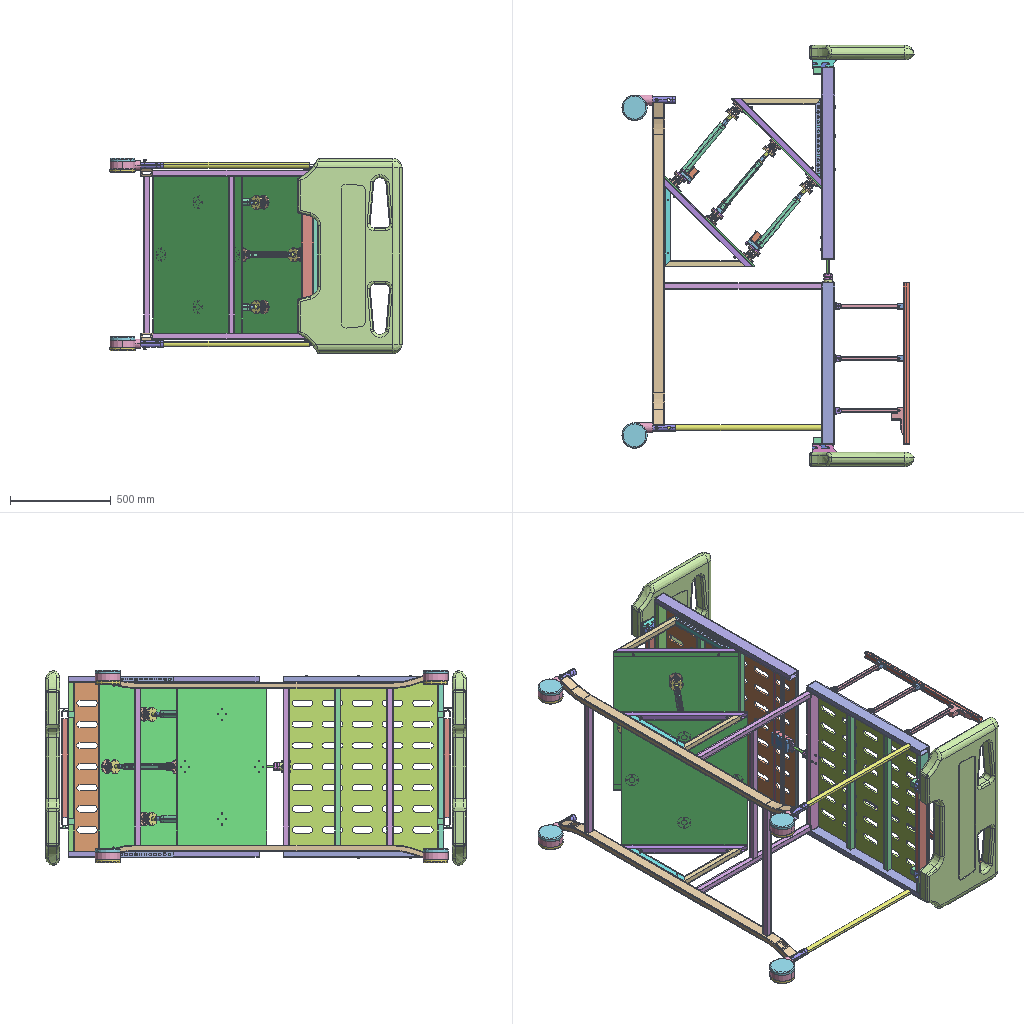Assembly | SolidWorks | 54 different items | 495 placed | box 1452 x 2094 x 971 mm
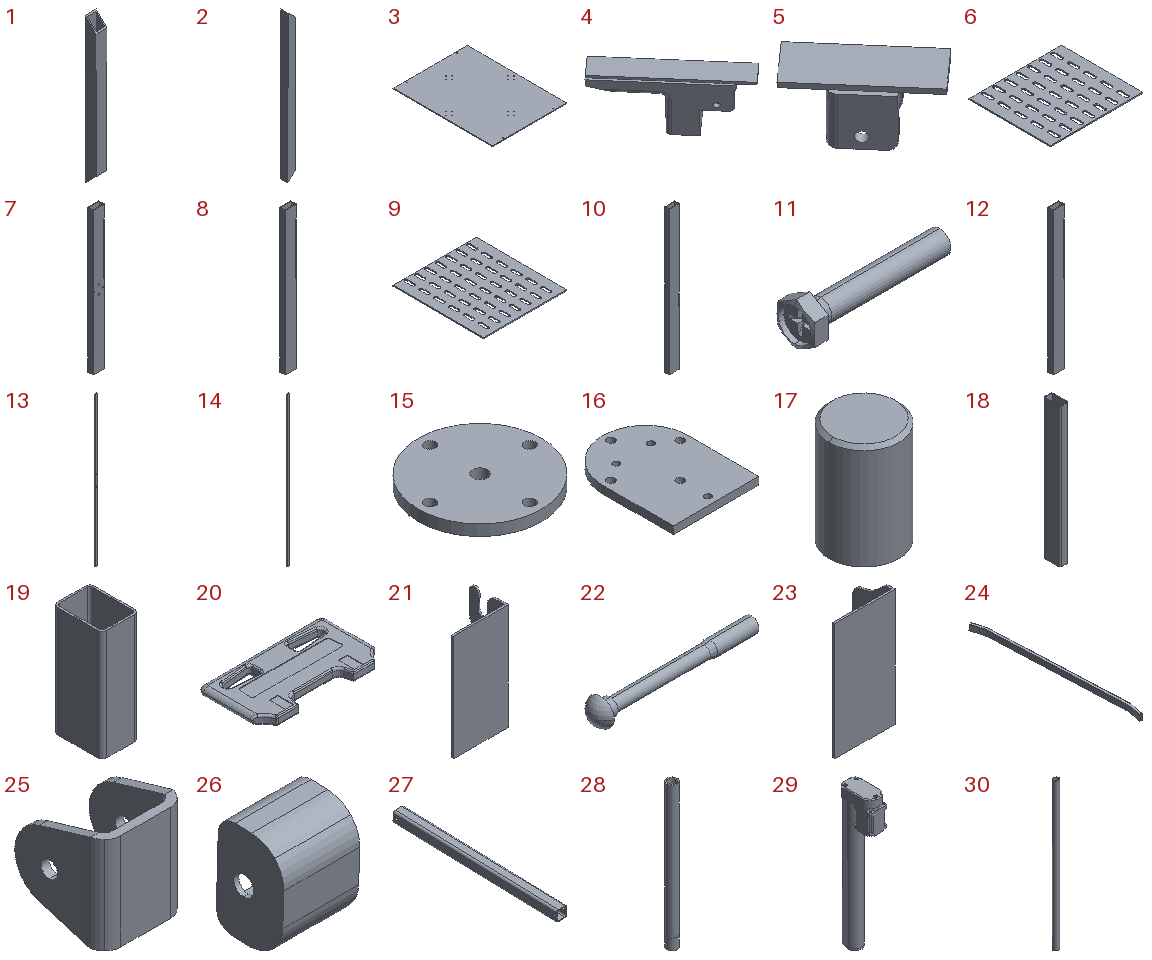Parts list (item | quantity | size | volume | features):
1 | x4 | 30 x 30 x 400 mm | 119880 mm3 | features ICE 3, Extrusion 1
2 | x4 | 30 x 30 x 625.685 mm | 192663 mm3 | features Cut 2, Extrusion 1, ICE 1
3 | x2 | 625.685 x 840 x 6 mm | 3151419 mm3 | features Cut 2, Extrusion 1
4 | x2 | 118.942 x 131.952 x 65.78 mm | 109548 mm3 | features BaseBody 1
5 | x4 | 64.897 x 69.371 x 35.986 mm | 22135 mm3 | features BaseBody 1
6 | x1 | 840 x 740 x 10 mm | 5160574 mm3 | features Extrusion 1, ICE 1
7 | x1 | 65 x 30 x 840 mm | 447881 mm3 | features ICE 2, Extrusion 1
8 | x1 | 65 x 30 x 840 mm | 448560 mm3 | features Extrusion 1, ICE 1
9 | x1 | 840 x 920 x 10 mm | 6461489 mm3 | features Extrusion 1, ICE 1
10 | x2 | 65 x 30 x 950 mm | 506395 mm3 | features Cut 1, Extrusion 1, ICE 1
11 | x24 | 39 x 10 x 11.547 mm | 1217 mm3 | features Cut 2, RevCut 2, CirPattern 1, Extrusion 1, LPattern 1, Revolution 1
12 | x1 | 65 x 30 x 840 mm | 448560 mm3 | features Extrusion 1, ICE 1
13 | x2 | 12 x 3 x 840 mm | 21761 mm3 | features 3DProfileFeature 1, Extrusion 1, HoleWzd 1, ICE 1
14 | x2 | 12 x 3 x 840 mm | 21840 mm3 | features Extrusion 1, ICE 1
15 | x4 | 68 x 68 x 6 mm | 21036 mm3 | features ICE 2, Extrusion 1
16 | x4 | 68 x 89.927 x 6 mm | 32907 mm3 | features Cut 2, Extrusion 1
17 | x8 | 10 x 10 x 15 mm | 1174 mm3 | features BaseBody 1
18 | x2 | 30 x 60 x 490 mm | 161830 mm3 | features BaseBody 1
19 | x4 | 30 x 40 x 90 mm | 17395 mm3 | features BaseBody 1
20 | x2 | 970 x 520 x 70 mm | 26489318 mm3 | features BaseBody 1
21 | x2 | 62 x 42 x 120 mm | 21824 mm3 | features BaseBody 1
22 | x6 | 85.28 x 14.328 x 14.328 mm | 3773 mm3 | features RevCut 2, LPattern 1, Revolution 1, Rib 1
23 | x2 | 62 x 42 x 120 mm | 21824 mm3 | features BaseBody 1
24 | x2 | 248.187 x 1610 x 188.463 mm | 531554 mm3 | features BaseBody 1
25 | x6 | 30 x 32.5 x 35 mm | 7224 mm3 | features BaseBody 1
26 | x6 | 23 x 20.424 x 30.136 mm | 5420 mm3 | features BaseBody 1
27 | x6 | 20 x 310.443 x 28.789 mm | 31845 mm3 | features BaseBody 1
28 | x4 | 20 x 20 x 284 mm | 37985 mm3 | features BaseBody 2
29 | x4 | 40 x 75.927 x 328 mm | 216478 mm3 | features BaseBody 20
30 | x2 | 28.9 x 28.9 x 840 mm | 105036 mm3 | features Extrusion 1
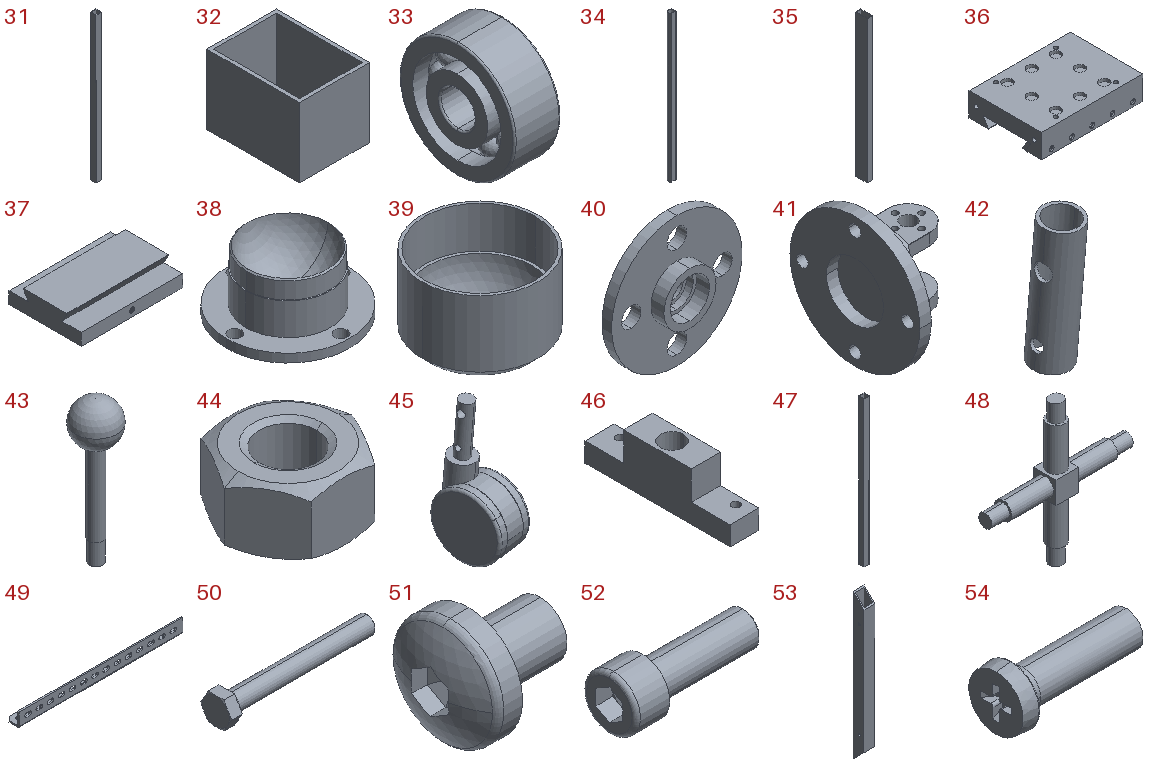31 | x5 | 30 x 30 x 784 mm | 254016 mm3 | features Extrusion 1
32 | x4 | 30 x 40 x 30 mm | 6030 mm3 | features Extrusion 1, ICE 1
33 | x32 | 4 x 10 x 10 mm | 208.039 mm3 | features Revolution 3, CirPattern 1, Fillet 1
34 | x2 | 30 x 30 x 800 mm | 132921 mm3 | features ICE 2, Extrusion 1
35 | x2 | 30 x 65 x 800 mm | 427200 mm3 | features Extrusion 1, ICE 1
36 | x1 | 105 x 75 x 24.5 mm | 146432 mm3 | features BaseBody 7, ICE 2
37 | x1 | 105 x 74.5 x 22 mm | 135687 mm3 | features BaseBody 1
38 | x1 | 58 x 58 x 27.375 mm | 26425 mm3 | features ICE 2, Extrusion 1, RevCut 1, StudWizard 1
39 | x1 | 42 x 42 x 27 mm | 6192 mm3 | features ICE 5, Chamfer 1, Extrusion 1, RevCut 1
40 | x32 | 20 x 3.5 x 20 mm | 446.892 mm3 | features ICE 1, Revolution 1
41 | x16 | 39 x 68 x 68 mm | 29102 mm3 | features ICE 8, MirrorPattern 2, Revolution 1
42 | x4 | 34.667 x 42.72 x 117.323 mm | 30652 mm3 | features BaseBody 1
43 | x1 | 38 x 38 x 130 mm | 40616 mm3 | features Revolution 2, StudWizard 1
44 | x33 | 9.238 x 8 x 4.7 mm | 190.603 mm3 | features RevCut 2, Chamfer 1, Extrusion 1, LPattern 1
45 | x4 | 83.862 x 131.58 x 256.05 mm | 967710 mm3 | features BaseBody 3
46 | x1 | 15 x 75 x 25 mm | 16595 mm3 | features Cut 3, Extrusion 1
47 | x4 | 30 x 30 x 840 mm | 272160 mm3 | features Extrusion 1, ICE 1
48 | x8 | 32 x 5 x 32 mm | 715.619 mm3 | features ICE 4, MirrorPattern 4, Extrusion 1
49 | x2 | 352 x 30 x 30 mm | 51066 mm3 | features ICE 3, Cut 1, Extrusion 1, Fillet 1
50 | x4 | 43.65 x 8.984 x 7.78 mm | 971.133 mm3 | features RevCut 3, Boss 1, Chamfer 1, Extrusion 1, Fillet 1, LPattern 1
51 | x4 | 12.382 x 12 x 12 mm | 602.281 mm3 | features Cut 2, Fillet 2, RevCut 2, Boss 1, Extrusion 1, LPattern 1
52 | x212 | 40 x 16 x 16 mm | 4032 mm3 | features Fillet 2, RevCut 2, Boss 1, Chamfer 1, Cut 1, Extrusion 1, LPattern 1
53 | x4 | 30 x 30 x 400 mm | 119541 mm3 | features ICE 4, Extrusion 1
54 | x2 | 11.4 x 4.982 x 4.982 mm | 94.532 mm3 | features Draft 2, Fillet 2, Boss 1, Cut 1, Extrusion 1, LPattern 1, PLine 1, RevCut 1
Mates (type | each side: item.copy, entity, surface, feature), first 538 of 1066 lines:
Coincident | 8.1 face plane Boss-Extrude1 | 35.1 face plane Boss-Extrude1 | 3 times
Coincident | 8.1 face plane Boss-Extrude1 | 35.2 face plane Boss-Extrude1 | 2 times
Coincident | 35.1 face plane Boss-Extrude1 | 35.2 face plane Boss-Extrude1
Coincident | 35.1 face plane Boss-Extrude1 | 47.1 face plane Boss-Extrude1
DistanceDim | 47.1 face plane Boss-Extrude1 | 35.1 face plane Boss-Extrude1
Coincident | 47.1 face plane Boss-Extrude1 | 47.2 face plane Boss-Extrude1
Coincident | 35.1 face plane Boss-Extrude1 | 47.2 face plane Boss-Extrude1
Coincident | 35.1 face plane Boss-Extrude1 | 7.1 face plane Boss-Extrude1 | 3 times
DistanceDim | 47.2 face plane Boss-Extrude1 | 7.1 face plane Boss-Extrude1
DistanceDim | 47.1 face plane Boss-Extrude1 | 8.1 face plane Boss-Extrude1
Coincident | 35.1 face plane Boss-Extrude1 | 25.1 face plane Guardrail support connector seat1^Guardrail bottom beam-6-solid1 | 2 times
DistanceDim | 25.1 face plane Guardrail support connector seat1^Guardrail bottom beam-6-solid1 | 8.1 face plane Boss-Extrude1
Coincident | 35.1 face plane Boss-Extrude1 | 25.2 face plane Guardrail support connector seat1^Guardrail bottom beam-6-solid1 | 2 times
DistanceDim | 25.2 face plane Guardrail support connector seat1^Guardrail bottom beam-6-solid1 | 8.1 face plane Boss-Extrude1
Coincident | 35.1 face plane Boss-Extrude1 | 25.3 face plane Guardrail support connector seat1^Guardrail bottom beam-6-solid1 | 2 times
DistanceDim | 25.3 face plane Guardrail support connector seat1^Guardrail bottom beam-6-solid1 | 8.1 face plane Boss-Extrude1
Coincident | 35.2 face plane Boss-Extrude1 | 25.4 face plane Guardrail support connector seat1^Guardrail bottom beam-6-solid1 | 2 times
Coincident | 25.1 face plane Guardrail support connector seat1^Guardrail bottom beam-6-solid1 | 25.4 face plane Guardrail support connector seat1^Guardrail bottom beam-6-solid1
Coincident | 35.2 face plane Boss-Extrude1 | 25.5 face plane Guardrail support connector seat1^Guardrail bottom beam-6-solid1 | 2 times
Coincident | 35.2 face plane Boss-Extrude1 | 25.6 face plane Guardrail support connector seat1^Guardrail bottom beam-6-solid1 | 2 times
Coincident | 25.2 face plane Guardrail support connector seat1^Guardrail bottom beam-6-solid1 | 25.5 face plane Guardrail support connector seat1^Guardrail bottom beam-6-solid1
Coincident | 25.3 face plane Guardrail support connector seat1^Guardrail bottom beam-6-solid1 | 25.6 face plane Guardrail support connector seat1^Guardrail bottom beam-6-solid1
Concentric | 25.1 face cylinder Guardrail support connector seat1^Guardrail bottom beam-6-solid1 | 26.1 face cylinder Nylon seat1^Guardrail assembly-6-solid1
Parallel | 25.1 face plane Guardrail support connector seat1^Guardrail bottom beam-6-solid1 | 26.1 face plane Nylon seat1^Guardrail assembly-6-solid1
Coincident | 25.1 face plane Guardrail support connector seat1^Guardrail bottom beam-6-solid1 | 26.1 face plane Nylon seat1^Guardrail assembly-6-solid1
Concentric | 25.2 face cylinder Guardrail support connector seat1^Guardrail bottom beam-6-solid1 | 26.2 face cylinder Nylon seat1^Guardrail assembly-6-solid1
Parallel | 25.2 face plane Guardrail support connector seat1^Guardrail bottom beam-6-solid1 | 26.2 face plane Nylon seat1^Guardrail assembly-6-solid1
Coincident | 25.2 face plane Guardrail support connector seat1^Guardrail bottom beam-6-solid1 | 26.2 face plane Nylon seat1^Guardrail assembly-6-solid1
Concentric | 25.3 face cylinder Guardrail support connector seat1^Guardrail bottom beam-6-solid1 | 26.3 face cylinder Nylon seat1^Guardrail assembly-6-solid1
Parallel | 25.3 face plane Guardrail support connector seat1^Guardrail bottom beam-6-solid1 | 26.3 face plane Nylon seat1^Guardrail assembly-6-solid1
Coincident | 25.3 face plane Guardrail support connector seat1^Guardrail bottom beam-6-solid1 | 26.3 face plane Nylon seat1^Guardrail assembly-6-solid1
Concentric | 25.4 face cylinder Guardrail support connector seat1^Guardrail bottom beam-6-solid1 | 26.4 face cylinder Nylon seat1^Guardrail assembly-6-solid1
Parallel | 25.4 face plane Guardrail support connector seat1^Guardrail bottom beam-6-solid1 | 26.4 face plane Nylon seat1^Guardrail assembly-6-solid1
Coincident | 25.4 face plane Guardrail support connector seat1^Guardrail bottom beam-6-solid1 | 26.4 face plane Nylon seat1^Guardrail assembly-6-solid1
Concentric | 25.5 face cylinder Guardrail support connector seat1^Guardrail bottom beam-6-solid1 | 26.5 face cylinder Nylon seat1^Guardrail assembly-6-solid1
Parallel | 25.5 face plane Guardrail support connector seat1^Guardrail bottom beam-6-solid1 | 26.5 face plane Nylon seat1^Guardrail assembly-6-solid1
Coincident | 25.5 face plane Guardrail support connector seat1^Guardrail bottom beam-6-solid1 | 26.5 face plane Nylon seat1^Guardrail assembly-6-solid1
Concentric | 25.6 face cylinder Guardrail support connector seat1^Guardrail bottom beam-6-solid1 | 26.6 face cylinder Nylon seat1^Guardrail assembly-6-solid1
Parallel | 25.6 face plane Guardrail support connector seat1^Guardrail bottom beam-6-solid1 | 26.6 face plane Nylon seat1^Guardrail assembly-6-solid1
Coincident | 25.6 face plane Guardrail support connector seat1^Guardrail bottom beam-6-solid1 | 26.6 face plane Nylon seat1^Guardrail assembly-6-solid1
Concentric | 25.1 face cylinder Guardrail support connector seat1^Guardrail bottom beam-6-solid1 | 27.1 face cylinder Steel F 20x20x1.5-310 GB_T 6728-2002^Guardrail assembly-3-solid1
Parallel | 35.1 face plane Boss-Extrude1 | 27.1 face plane Steel F 20x20x1.5-310 GB_T 6728-2002^Guardrail assembly-3-solid1
Coincident | 26.1 face plane Nylon seat1^Guardrail assembly-6-solid1 | 27.1 face plane Steel F 20x20x1.5-310 GB_T 6728-2002^Guardrail assembly-3-solid1
Concentric | 25.2 face cylinder Guardrail support connector seat1^Guardrail bottom beam-6-solid1 | 27.2 face cylinder Steel F 20x20x1.5-310 GB_T 6728-2002^Guardrail assembly-3-solid1
Parallel | 35.1 face plane Boss-Extrude1 | 27.2 face plane Steel F 20x20x1.5-310 GB_T 6728-2002^Guardrail assembly-3-solid1
Coincident | 26.2 face plane Nylon seat1^Guardrail assembly-6-solid1 | 27.2 face plane Steel F 20x20x1.5-310 GB_T 6728-2002^Guardrail assembly-3-solid1
Concentric | 25.3 face cylinder Guardrail support connector seat1^Guardrail bottom beam-6-solid1 | 27.3 face cylinder Steel F 20x20x1.5-310 GB_T 6728-2002^Guardrail assembly-3-solid1
Parallel | 35.1 face plane Boss-Extrude1 | 27.3 face plane Steel F 20x20x1.5-310 GB_T 6728-2002^Guardrail assembly-3-solid1
Coincident | 26.3 face plane Nylon seat1^Guardrail assembly-6-solid1 | 27.3 face plane Steel F 20x20x1.5-310 GB_T 6728-2002^Guardrail assembly-3-solid1
Concentric | 25.4 face cylinder Guardrail support connector seat1^Guardrail bottom beam-6-solid1 | 27.4 face cylinder Steel F 20x20x1.5-310 GB_T 6728-2002^Guardrail assembly-3-solid1
Parallel | 35.2 face plane Boss-Extrude1 | 27.4 face plane Steel F 20x20x1.5-310 GB_T 6728-2002^Guardrail assembly-3-solid1
Concentric | 25.5 face cylinder Guardrail support connector seat1^Guardrail bottom beam-6-solid1 | 27.5 face cylinder Steel F 20x20x1.5-310 GB_T 6728-2002^Guardrail assembly-3-solid1
Parallel | 35.2 face plane Boss-Extrude1 | 27.5 face plane Steel F 20x20x1.5-310 GB_T 6728-2002^Guardrail assembly-3-solid1
Coincident | 26.5 face plane Nylon seat1^Guardrail assembly-6-solid1 | 27.5 face plane Steel F 20x20x1.5-310 GB_T 6728-2002^Guardrail assembly-3-solid1
Concentric | 26.6 face cylinder Nylon seat1^Guardrail assembly-6-solid1 | 27.6 face cylinder Steel F 20x20x1.5-310 GB_T 6728-2002^Guardrail assembly-3-solid1
Parallel | 35.2 face plane Boss-Extrude1 | 27.6 face plane Steel F 20x20x1.5-310 GB_T 6728-2002^Guardrail assembly-3-solid1
Coincident | 26.6 face plane Nylon seat1^Guardrail assembly-6-solid1 | 27.6 face plane Steel F 20x20x1.5-310 GB_T 6728-2002^Guardrail assembly-3-solid1
Concentric | 27.4 face cylinder Steel F 20x20x1.5-310 GB_T 6728-2002^Guardrail assembly-3-solid1 | 4.1 face cylinder Nylon seat3^Upper crossbeam assembly-1-solid1
Parallel | 35.2 face plane Boss-Extrude1 | 4.1 face plane Nylon seat3^Upper crossbeam assembly-1-solid1
Coincident | 27.4 face plane Steel F 20x20x1.5-310 GB_T 6728-2002^Guardrail assembly-3-solid1 | 4.1 face plane Nylon seat3^Upper crossbeam assembly-1-solid1
Coincident | 26.4 face plane Nylon seat1^Guardrail assembly-6-solid1 | 27.4 face plane Steel F 20x20x1.5-310 GB_T 6728-2002^Guardrail assembly-3-solid1
Concentric | 27.1 face cylinder Steel F 20x20x1.5-310 GB_T 6728-2002^Guardrail assembly-3-solid1 | 4.2 face cylinder Nylon seat3^Upper crossbeam assembly-1-solid1
Parallel | 35.1 face plane Boss-Extrude1 | 4.2 face plane Nylon seat3^Upper crossbeam assembly-1-solid1
Coincident | 27.1 face plane Steel F 20x20x1.5-310 GB_T 6728-2002^Guardrail assembly-3-solid1 | 4.2 face plane Nylon seat3^Upper crossbeam assembly-1-solid1
Concentric | 27.5 face cylinder Steel F 20x20x1.5-310 GB_T 6728-2002^Guardrail assembly-3-solid1 | 5.1 face cylinder Nylon seat2^Upper crossbeam assembly-4-solid1
Parallel | 35.2 face plane Boss-Extrude1 | 5.1 face plane Nylon seat2^Upper crossbeam assembly-4-solid1
Coincident | 27.5 face plane Steel F 20x20x1.5-310 GB_T 6728-2002^Guardrail assembly-3-solid1 | 5.1 face plane Nylon seat2^Upper crossbeam assembly-4-solid1
Concentric | 27.6 face cylinder Steel F 20x20x1.5-310 GB_T 6728-2002^Guardrail assembly-3-solid1 | 5.2 face cylinder Nylon seat2^Upper crossbeam assembly-4-solid1
Parallel | 35.2 face plane Boss-Extrude1 | 5.2 face plane Nylon seat2^Upper crossbeam assembly-4-solid1
Coincident | 27.6 face plane Steel F 20x20x1.5-310 GB_T 6728-2002^Guardrail assembly-3-solid1 | 5.2 face plane Nylon seat2^Upper crossbeam assembly-4-solid1
Concentric | 27.2 face cylinder Steel F 20x20x1.5-310 GB_T 6728-2002^Guardrail assembly-3-solid1 | 5.3 face cylinder Nylon seat2^Upper crossbeam assembly-4-solid1
Parallel | 35.1 face plane Boss-Extrude1 | 5.3 face plane Nylon seat2^Upper crossbeam assembly-4-solid1
Coincident | 27.2 face plane Steel F 20x20x1.5-310 GB_T 6728-2002^Guardrail assembly-3-solid1 | 5.3 face plane Nylon seat2^Upper crossbeam assembly-4-solid1
Concentric | 27.3 face cylinder Steel F 20x20x1.5-310 GB_T 6728-2002^Guardrail assembly-3-solid1 | 5.4 face cylinder Nylon seat2^Upper crossbeam assembly-4-solid1
Parallel | 35.1 face plane Boss-Extrude1 | 5.4 face plane Nylon seat2^Upper crossbeam assembly-4-solid1
Coincident | 27.3 face plane Steel F 20x20x1.5-310 GB_T 6728-2002^Guardrail assembly-3-solid1 | 5.4 face plane Nylon seat2^Upper crossbeam assembly-4-solid1
Coincident | 4.2 face plane Nylon seat3^Upper crossbeam assembly-1-solid1 | 34.1 face plane Cut-Extrude2 | 2 times
Coincident | 35.1 face plane Boss-Extrude1 | 34.1 face plane Boss-Extrude1
Coincident | 4.1 face plane Nylon seat3^Upper crossbeam assembly-1-solid1 | 34.2 face plane Cut-Extrude2 | 2 times
Coincident | 35.2 face plane Boss-Extrude1 | 34.2 face plane Boss-Extrude1
Concentric | 5.4 face cylinder Nylon seat2^Upper crossbeam assembly-4-solid1 | 11.1 face cylinder Revolve1
Coincident | 5.4 face plane Nylon seat2^Upper crossbeam assembly-4-solid1 | 11.1 face plane BaseHead
Concentric | 25.3 face cylinder Guardrail support connector seat1^Guardrail bottom beam-6-solid1 | 11.2 face cylinder Revolve1
Coincident | 25.3 face plane Guardrail support connector seat1^Guardrail bottom beam-6-solid1 | 11.2 face plane BaseHead
Concentric | 25.2 face cylinder Guardrail support connector seat1^Guardrail bottom beam-6-solid1 | 11.3 face cylinder Revolve1
Concentric | 5.3 face cylinder Nylon seat2^Upper crossbeam assembly-4-solid1 | 11.4 face cylinder Revolve1
Concentric | 25.1 face cylinder Guardrail support connector seat1^Guardrail bottom beam-6-solid1 | 11.5 face cylinder Revolve1
Concentric | 4.2 face cylinder Nylon seat3^Upper crossbeam assembly-1-solid1 | 11.6 face cylinder Revolve1
Coincident | 25.2 face plane Guardrail support connector seat1^Guardrail bottom beam-6-solid1 | 11.3 face plane BaseHead
Coincident | 5.3 face plane Nylon seat2^Upper crossbeam assembly-4-solid1 | 11.4 face plane BaseHead
Coincident | 25.1 face plane Guardrail support connector seat1^Guardrail bottom beam-6-solid1 | 11.5 face plane BaseHead
Coincident | 4.2 face plane Nylon seat3^Upper crossbeam assembly-1-solid1 | 11.6 face plane BaseHead
Concentric | 25.6 face cylinder Guardrail support connector seat1^Guardrail bottom beam-6-solid1 | 11.7 face cylinder Revolve1
Coincident | 25.6 face plane Guardrail support connector seat1^Guardrail bottom beam-6-solid1 | 11.7 face plane BaseHead
Concentric | 5.2 face cylinder Nylon seat2^Upper crossbeam assembly-4-solid1 | 11.8 face cylinder Revolve1
Coincident | 5.2 face plane Nylon seat2^Upper crossbeam assembly-4-solid1 | 11.8 face plane BaseHead
Concentric | 25.5 face cylinder Guardrail support connector seat1^Guardrail bottom beam-6-solid1 | 11.9 face cylinder Revolve1
Coincident | 25.5 face plane Guardrail support connector seat1^Guardrail bottom beam-6-solid1 | 11.9 face plane BaseHead
Concentric | 5.1 face cylinder Nylon seat2^Upper crossbeam assembly-4-solid1 | 11.10 face cylinder Revolve1
Coincident | 5.1 face plane Nylon seat2^Upper crossbeam assembly-4-solid1 | 11.10 face plane BaseHead
Concentric | 4.1 face cylinder Nylon seat3^Upper crossbeam assembly-1-solid1 | 11.11 face cylinder Revolve1
Coincident | 4.1 face plane Nylon seat3^Upper crossbeam assembly-1-solid1 | 11.11 face plane BaseHead
Concentric | 25.4 face cylinder Guardrail support connector seat1^Guardrail bottom beam-6-solid1 | 11.12 face cylinder Revolve1
Coincident | 25.4 face plane Guardrail support connector seat1^Guardrail bottom beam-6-solid1 | 11.12 face plane BaseHead
Concentric | 11.7 face cylinder Revolve1 | 44.1 face cylinder BaseNut
Concentric | 11.8 face cylinder Revolve1 | 44.2 face cylinder BaseNut
Concentric | 11.9 face cylinder Revolve1 | 44.3 face cylinder BaseNut
Concentric | 11.10 face cylinder Revolve1 | 44.4 face cylinder BaseNut
Concentric | 11.12 face cylinder Revolve1 | 44.5 face cylinder BaseNut
Concentric | 11.11 face cylinder Revolve1 | 44.6 face cylinder BaseNut
Coincident | 25.4 face plane Guardrail support connector seat1^Guardrail bottom beam-6-solid1 | 44.5 face plane BaseNut
Coincident | 4.1 face plane Nylon seat3^Upper crossbeam assembly-1-solid1 | 44.6 face plane BaseNut
Coincident | 5.1 face plane Nylon seat2^Upper crossbeam assembly-4-solid1 | 44.4 face plane BaseNut
Coincident | 25.5 face plane Guardrail support connector seat1^Guardrail bottom beam-6-solid1 | 44.3 face plane BaseNut
Coincident | 25.6 face plane Guardrail support connector seat1^Guardrail bottom beam-6-solid1 | 44.1 face plane BaseNut
Concentric | 11.1 face cylinder Revolve1 | 44.7 face cylinder BaseNut
Concentric | 11.4 face cylinder Revolve1 | 44.8 face cylinder BaseNut
Concentric | 11.6 face cylinder Revolve1 | 44.9 face cylinder BaseNut
Coincident | 4.2 face plane Nylon seat3^Upper crossbeam assembly-1-solid1 | 44.9 face plane BaseNut
Concentric | 11.5 face cylinder Revolve1 | 44.10 face cylinder BaseNut
Coincident | 25.1 face plane Guardrail support connector seat1^Guardrail bottom beam-6-solid1 | 44.10 face plane BaseNut
Concentric | 11.3 face cylinder Revolve1 | 44.11 face cylinder BaseNut
Coincident | 5.3 face plane Nylon seat2^Upper crossbeam assembly-4-solid1 | 44.8 face plane BaseNut
Coincident | 25.2 face plane Guardrail support connector seat1^Guardrail bottom beam-6-solid1 | 44.11 face plane BaseNut
Concentric | 11.2 face cylinder Revolve1 | 44.12 face cylinder BaseNut
Coincident | 25.3 face plane Guardrail support connector seat1^Guardrail bottom beam-6-solid1 | 44.12 face plane BaseNut
Coincident | 5.4 face plane Nylon seat2^Upper crossbeam assembly-4-solid1 | 44.7 face plane BaseNut
Coincident | 7.1 face plane Boss-Extrude1 | 38.1 face plane Boss-Extrude1
Concentric | 7.1 face cylinder Cut-Extrude3 | 38.1 face cylinder Cut-Extrude1 | 2 times
Concentric | 38.1 face sphere Cut-Revolve4 | 43.1 face sphere Revolve5
Concentric | 38.1 face cylinder Boss-Extrude2 | 43.1 face cylinder Revolve6
Concentric | 38.1 face cylinder Boss-Extrude2 | 39.1 face cylinder Boss-Extrude1
Coincident | 38.1 face plane M39 mechanical thread stud1 | 39.1 face plane Boss-Extrude1
Concentric | 43.1 face cylinder Revolve6 | 46.1 face cylinder Cut-Extrude3
Coincident | 43.1 face plane M12x1.25 mechanical thread stud1 | 46.1 face plane Boss-Extrude1
Concentric | 46.1 face cylinder Cut-Extrude1 | 36.1 face cylinder 21060_TOP^COMPANY_A_21060-075105.step-1-solid1 | 2 times
Coincident | 46.1 face plane Boss-Extrude1 | 36.1 face plane 21060_TOP^COMPANY_A_21060-075105.step-1-solid1
Lock | 10.1 select_type:0 | 12.1 select_type:0
Lock | 10.2 select_type:0 | 12.1 select_type:0
Coincident | 37.1 face plane 21060_BOTTOM^COMPANY_A_21060-075105.step-1-solid1 | 36.1 face plane 21060_TOP^COMPANY_A_21060-075105.step-1-solid1 | 2 times
Coincident | 37.1 face plane 21060_BOTTOM^COMPANY_A_21060-075105.step-1-solid1 | 36.1 face plane 21060_TOP^COMPANY_A_21060-075105.step-1-solid2
Parallel | 7.1 face plane Boss-Extrude1 | 36.1 face plane Boss-Extrude1
Coincident | 10.2 face plane Boss-Extrude1 | 46.1 face plane Boss-Extrude1
Coincident | 35.1 face plane Boss-Extrude1 | 10.2 face plane Boss-Extrude1 | 2 times
Concentric | 37.1 face cylinder 21060_BOTTOM^COMPANY_A_21060-075105.step-1-solid1 | 13.1 face cylinder M6 Tapped Hole1 | 2 times
Coincident | 10.1 face plane Boss-Extrude1 | 13.1 face plane Boss-Extrude1
Concentric | 37.1 face cylinder 21060_BOTTOM^COMPANY_A_21060-075105.step-1-solid1 | 13.2 face cylinder M6 Tapped Hole1 | 2 times
Coincident | 10.2 face plane Boss-Extrude1 | 13.2 face plane Boss-Extrude1
Coincident | 10.2 face plane Boss-Extrude1 | 47.3 face plane Boss-Extrude1
DistanceDim | 47.3 face plane Boss-Extrude1 | 10.2 face plane Boss-Extrude1
Coincident | 10.2 face plane Boss-Extrude1 | 47.4 face plane Boss-Extrude1
DistanceDim | 47.4 face plane Boss-Extrude1 | 10.2 face plane Boss-Extrude1
DistanceDim | 47.3 face plane Boss-Extrude1 | 12.1 face plane Boss-Extrude1
DistanceDim | 47.4 face plane Boss-Extrude1 | 37.1 face plane 21060_BOTTOM^COMPANY_A_21060-075105.step-1-solid1
Coincident | 20.1 face plane Input1 | 21.1 face plane Input1 | 3 times
Coincident | 20.1 face plane Input1 | 23.1 face plane Input1 | 3 times
Concentric | 23.1 face cylinder Input1 | 17.1 face cylinder Input1
Coincident | 23.1 face plane Input1 | 17.1 face plane Input1
Concentric | 23.1 face cylinder Input1 | 17.2 face cylinder Input1
Coincident | 17.2 face plane Input1 | 17.1 face plane Input1
Concentric | 21.1 face cylinder Input1 | 17.3 face cylinder Input1
Coincident | 21.1 face plane Input1 | 17.3 face plane Input1
DistanceDim | 19.1 face plane Input1 | 21.1 face plane Input1 | 2 times
Concentric | 21.1 face cylinder Input1 | 17.4 face cylinder Input1
Coincident | 17.3 face plane Input1 | 17.4 face plane Input1
Coincident | 19.1 face plane Input1 | 19.2 face plane Input1
Coincident | 19.1 face plane Input1 | 18.1 face plane Input1 | 3 times
Coincident | 18.1 face plane Input1 | 19.2 face plane Input1 | 2 times
Coincident | 20.1 face plane Input1 | 19.1 face plane Input1
DistanceDim | 19.2 face plane Input1 | 18.1 face plane Input1
Coincident | 23.2 face plane Input1 | 20.2 face plane Input1 | 3 times
Coincident | 21.2 face plane Input1 | 20.2 face plane Input1 | 3 times
DistanceDim | 19.3 face plane Input1 | 21.2 face plane Input1 | 2 times
Concentric | 17.5 face cylinder Input1 | 23.2 face cylinder Input1
Concentric | 17.6 face cylinder Input1 | 21.2 face cylinder Input1
Concentric | 17.7 face cylinder Input1 | 23.2 face cylinder Input1
Concentric | 17.8 face cylinder Input1 | 21.2 face cylinder Input1
DistanceDim | 19.4 face plane Input1 | 18.2 face plane Input1
Coincident | 18.2 face plane Input1 | 19.3 face plane Input1 | 3 times
Coincident | 19.4 face plane Input1 | 19.3 face plane Input1
Coincident | 17.6 face plane Input1 | 17.8 face plane Input1
Coincident | 18.2 face plane Input1 | 19.4 face plane Input1 | 2 times
Coincident | 19.3 face plane Input1 | 20.2 face plane Input1
Coincident | 17.7 face plane Input1 | 17.5 face plane Input1
Coincident | 17.5 face plane Input1 | 23.2 face plane Input1
Coincident | 17.8 face plane Input1 | 21.2 face plane Input1
Coincident | 19.3 face plane Input1 | 32.1 face plane Boss-Extrude1
Coincident | 19.3 edge | 32.1 face plane Boss-Extrude1
Coincident | 18.2 face plane Input1 | 32.1 face plane Boss-Extrude1
Coincident | 19.4 face plane Input1 | 32.2 face plane Boss-Extrude1
Coincident | 19.4 edge | 32.2 face plane Boss-Extrude1
Coincident | 32.1 face plane Boss-Extrude1 | 32.2 face plane Boss-Extrude1
Coincident | 8.1 face plane Boss-Extrude1 | 32.2 face plane Boss-Extrude1
Coincident | 8.1 face plane Boss-Extrude1 | 19.3 face plane Input1
DistanceDim | 21.2 face plane Input1 | 35.2 face plane Boss-Extrude1
Coincident | 19.1 face plane Input1 | 32.3 face plane Boss-Extrude1
Coincident | 19.1 edge | 32.3 face plane Boss-Extrude1
Coincident | 18.1 face plane Input1 | 32.3 face plane Boss-Extrude1
Coincident | 19.2 face plane Input1 | 32.4 face plane Boss-Extrude1
Coincident | 19.2 edge | 32.4 face plane Boss-Extrude1
Coincident | 32.3 face plane Boss-Extrude1 | 32.4 face plane Boss-Extrude1
Coincident | 12.1 face plane Boss-Extrude1 | 32.3 face plane Boss-Extrude1
Coincident | 32.1 face plane Boss-Extrude1 | 32.4 face plane Boss-Extrude1
Coincident | 12.1 face plane Boss-Extrude1 | 19.2 face plane Input1
Coincident | 10.2 face plane Boss-Extrude1 | 14.1 face plane Boss-Extrude1
Coincident | 13.2 face plane Boss-Extrude1 | 14.1 face plane Boss-Extrude1
Coincident | 10.2 face plane Boss-Extrude1 | 14.2 face plane Boss-Extrude1
Coincident | 10.1 face plane Boss-Extrude1 | 14.2 face plane Boss-Extrude1
Coincident | 10.2 face plane Boss-Extrude1 | 9.1 face plane Boss-Extrude1 | 2 times
Coincident | 12.1 face plane Boss-Extrude1 | 9.1 face plane Boss-Extrude1
Coincident | 35.1 face plane Boss-Extrude1 | 6.1 face plane Boss-Extrude1 | 2 times
Coincident | 7.1 face plane Boss-Extrude1 | 6.1 face plane Boss-Extrude1
Concentric | 38.1 face cylinder Cut-Extrude1 | 50.1 face cylinder BaseBody
Coincident | 38.1 face plane Boss-Extrude1 | 50.1 face plane BearingFace
Concentric | 38.1 face cylinder Cut-Extrude1 | 50.2 face cylinder BaseBody
Coincident | 50.1 face plane BaseHead | 50.2 face plane BaseHead
Concentric | 38.1 face cylinder Cut-Extrude1 | 50.3 face cylinder BaseBody
Coincident | 50.2 face plane BaseHead | 50.3 face plane BaseHead
Concentric | 38.1 face cylinder Cut-Extrude1 | 50.4 face cylinder BaseBody
Coincident | 50.1 face plane BaseHead | 50.4 face plane BaseHead
Coincident | 7.1 face plane Boss-Extrude1 | 44.13 face plane BaseNut
Concentric | 50.4 face cylinder BaseBody | 44.13 face cylinder BaseNut
Concentric | 50.2 face cylinder BaseBody | 44.14 face cylinder BaseNut
Coincident | 44.14 face plane BaseNut | 44.13 face plane BaseNut
Concentric | 50.3 face cylinder BaseBody | 44.15 face cylinder BaseNut
Coincident | 44.15 face plane BaseNut | 44.13 face plane BaseNut
Coincident | 13.1 face plane Boss-Extrude1 | 51.1 face plane BaseHead
Coincident | 13.1 face plane Boss-Extrude1 | 51.2 face plane BaseHead
Coincident | 13.2 face plane Boss-Extrude1 | 51.3 face plane BaseHead
Coincident | 13.2 face plane Boss-Extrude1 | 51.4 face plane BaseHead
Concentric | 13.1 face cylinder M6 Tapped Hole1 | 51.1 face cylinder BaseBody
Concentric | 13.1 edge | 51.2 face cylinder BaseHead
Concentric | 13.2 edge | 51.4 face cylinder BaseHead
Concentric | 13.2 face cylinder M6 Tapped Hole1 | 51.3 face cylinder BaseHead
Concentric | 46.1 face cylinder Cut-Extrude1 | 54.1 face cone SplitLine1
Coincident | 46.1 face plane Cut-Extrude2 | 54.1 face plane BaseHead
Coincident | 46.1 face plane Cut-Extrude2 | 54.2 face plane BaseHead
Concentric | 46.1 face cylinder Cut-Extrude1 | 54.2 face cylinder SplitLine1
Coincident | 10.2 face plane Boss-Extrude1 | 49.1 face plane Boss-Extrude2 | 2 times
Coincident | 53.1 face plane Cut-Extrude3 | 1.1 face plane Cut-Extrude6
Coincident | 53.1 face plane Boss-Extrude1 | 1.1 face plane Boss-Extrude1
Coincident | 53.1 face plane Boss-Extrude1 | 1.1 edge
Coincident | 53.1 face plane Cut-Extrude6 | 2.1 face plane Boss-Extrude1
Coincident | 1.1 face plane Cut-Extrude3 | 2.1 face plane Boss-Extrude1
Coincident | 1.1 face plane Boss-Extrude1 | 2.1 face plane Boss-Extrude1
Coincident | 1.1 face plane Boss-Extrude1 | 2.1 face plane Cut-Extrude2
Coincident | 49.1 face plane Boss-Extrude1 | 53.1 face plane Boss-Extrude1
Coincident | 10.2 face plane Boss-Extrude1 | 53.1 face plane Boss-Extrude1
Lock | 49.1 select_type:0 | 53.1 select_type:0
DistanceDim | 1.1 face plane Boss-Extrude1 | 12.1 face plane Boss-Extrude1
Coincident | 14.1 face plane Boss-Extrude1 | 9.1 face plane Boss-Extrude1
Coincident | 14.2 face plane Boss-Extrude1 | 9.1 face plane Boss-Extrude1
Coincident | 10.1 face plane Boss-Extrude1 | 49.2 face plane Boss-Extrude2 | 2 times
Coincident | 49.1 face plane Boss-Extrude1 | 49.2 face plane Boss-Extrude1
Coincident | 53.2 face plane Cut-Extrude6 | 1.2 face plane Cut-Extrude6
Coincident | 53.2 face plane Boss-Extrude1 | 1.2 edge
Coincident | 53.2 face plane Boss-Extrude1 | 1.2 face plane Boss-Extrude1
Coincident | 53.2 face plane Cut-Extrude3 | 2.2 face plane Boss-Extrude1
Coincident | 53.2 face plane Boss-Extrude1 | 2.2 face plane Boss-Extrude1
Coincident | 1.2 face plane Boss-Extrude1 | 2.2 face plane Cut-Extrude2
Coincident | 49.2 face plane Boss-Extrude1 | 53.2 face plane Boss-Extrude1
Coincident | 10.1 face plane Boss-Extrude1 | 53.2 face plane Boss-Extrude1
Coincident | 1.1 face plane Boss-Extrude1 | 1.2 face plane Boss-Extrude1
InPlace | 2.2 face plane Boss-Extrude1 | 3.1 plane
Concentric | 10.2 face cylinder Cut-Extrude2 | 22.1 face cylinder Base
Coincident | 10.2 face plane Boss-Extrude1 | 22.1 face plane Base
Concentric | 10.2 face cylinder Cut-Extrude2 | 22.2 face cylinder Cut-Revolve1
Concentric | 10.2 face cylinder Cut-Extrude2 | 22.3 face cylinder Cut-Revolve1
Concentric | 10.1 face cylinder Cut-Extrude2 | 22.4 face cylinder Cut-Revolve1
Concentric | 10.1 face cylinder Cut-Extrude2 | 22.5 face cylinder Cut-Revolve1
Concentric | 10.1 face cylinder Cut-Extrude2 | 22.6 face cylinder Cut-Revolve1
Coincident | 22.2 face plane Base | 22.1 face plane Base
Coincident | 22.2 face plane Base | 22.3 face plane Base
Coincident | 22.1 face plane Base | 22.5 face plane Base
Coincident | 22.5 face plane Base | 22.6 face plane Base
Coincident | 22.5 face plane Base | 22.4 face plane Base
Concentric | 22.2 face cylinder Base | 44.16 face cylinder BaseNut
Concentric | 10.1 face cylinder Cut-Extrude2 | 44.17 face cone EndChamfer
Coincident | 10.1 face plane Boss-Extrude1 | 44.17 face plane BaseNut
Concentric | 22.4 face cylinder Base | 44.18 face cylinder BaseNut
Concentric | 22.5 face cylinder Base | 44.19 face cylinder BaseNut
Concentric | 22.1 face cylinder Base | 44.20 face cylinder BaseNut
Concentric | 22.3 face cylinder Base | 44.21 face cylinder BaseNut
Concentric | 3.1 face cylinder Cut-Extrude2 | 11.13 face cylinder Revolve1
Coincident | 3.1 face plane Boss-Extrude1 | 11.13 face plane BaseHead
Concentric | 3.1 face cylinder Cut-Extrude2 | 11.14 face cylinder Revolve1
Coincident | 3.1 face plane Boss-Extrude1 | 11.14 face plane BaseHead
Concentric | 3.1 face cylinder Cut-Extrude2 | 11.15 face cylinder Revolve1
Coincident | 3.1 face plane Boss-Extrude1 | 11.15 face plane BaseHead
Concentric | 3.1 face cylinder Cut-Extrude2 | 11.16 face cylinder Revolve1
Coincident | 3.1 face plane Boss-Extrude1 | 11.16 face plane BaseHead
Concentric | 11.14 face cylinder Revolve1 | 44.22 face cylinder BaseNut
Concentric | 11.15 face cylinder Revolve1 | 44.23 face cylinder BaseNut
Concentric | 11.16 face cylinder Revolve1 | 44.24 face cylinder BaseNut
Concentric | 11.13 face cylinder Revolve1 | 44.25 face cylinder BaseNut
Coincident | 2.1 face plane Boss-Extrude1 | 44.25 face plane BaseNut
Coincident | 2.1 face plane Boss-Extrude1 | 44.22 face plane BaseNut
Coincident | 2.2 face plane Boss-Extrude1 | 44.23 face plane BaseNut
Coincident | 44.24 face plane BaseNut | 44.25 face plane BaseNut
Coincident | 49.1 face plane Boss-Extrude2 | 44.21 face plane BaseNut
Coincident | 44.16 face plane BaseNut | 44.21 face plane BaseNut
Coincident | 44.16 face plane BaseNut | 44.20 face plane BaseNut
Coincident | 49.2 face plane Boss-Extrude2 | 44.19 face plane BaseNut
Coincident | 44.18 face plane BaseNut | 44.19 face plane BaseNut
Concentric | 49.1 face cylinder Cut-Extrude2 | 11.17 face cylinder Revolve1
Coincident | 49.2 face plane Boss-Extrude1 | 11.18 face plane BaseHead
Coincident | 49.2 face plane Boss-Extrude1 | 11.19 face plane BaseHead
Concentric | 53.2 face cylinder Cut-Extrude7 | 11.19 face cone Revolve1
Concentric | 53.2 face cylinder Cut-Extrude7 | 11.18 face cone Revolve1
Coincident | 49.1 face plane Boss-Extrude1 | 11.17 face plane BaseHead
Coincident | 49.1 face plane Boss-Extrude1 | 11.20 face plane BaseHead
Concentric | 53.1 face cylinder Cut-Extrude7 | 11.20 face cylinder Revolve1
Coincident | 53.2 face plane Boss-Extrude1 | 44.26 face plane BaseNut
Coincident | 53.2 face plane Boss-Extrude1 | 44.27 face plane BaseNut
Concentric | 11.18 face cylinder Revolve1 | 44.26 face cylinder BaseNut
Concentric | 11.19 face cylinder Revolve1 | 44.27 face cylinder BaseNut
Coincident | 53.1 face plane Boss-Extrude1 | 44.28 face plane BaseNut
Concentric | 53.1 face cylinder Cut-Extrude7 | 44.29 face cone EndChamfer
Coincident | 53.1 face plane Boss-Extrude1 | 44.29 face plane BaseNut
Concentric | 11.20 face cylinder Revolve1 | 44.28 face cylinder BaseNut
Concentric | 48.1 face cylinder Cut-Extrude1 | 33.1 face cylinder Revolve2
Coincident | 48.1 face plane Cut-Extrude1 | 33.1 face plane Revolve2
Concentric | 48.1 face cylinder Mirror3 | 33.2 face cylinder Revolve2
Coincident | 48.1 face plane Mirror3 | 33.2 face plane Revolve2
Concentric | 48.1 face cylinder Cut-Extrude2 | 33.3 face cylinder Revolve2
Coincident | 48.1 face plane Cut-Extrude2 | 33.3 face plane Revolve2
Concentric | 48.1 face cylinder Mirror4 | 33.4 face cylinder Revolve2
Coincident | 48.1 face plane Mirror4 | 33.4 face plane Revolve2
Concentric | 41.1 face cylinder Cut-Extrude1 | 48.1 face cylinder Mirror2
DistanceDim | 33.3 face plane Revolve2 | 41.1 face plane Cut-Extrude3
Concentric | 41.2 face cylinder Cut-Extrude1 | 48.1 face cylinder Boss-Extrude2
DistanceDim | 33.1 face plane Revolve2 | 41.2 face plane Cut-Extrude3
Concentric | 41.1 face cylinder Cut-Extrude1 | 40.1 face cylinder Revolve1
Coincident | 41.1 face plane Mirror1 | 40.1 face plane Revolve1
Concentric | 41.1 face cylinder Cut-Extrude7 | 40.1 face cylinder Cut-Extrude1
Concentric | 40.1 face cylinder Cut-Extrude1 | 52.1 face cylinder BaseBody
Coincident | 40.1 face plane Revolve1 | 52.1 face plane BaseHead
Concentric | 41.1 face cylinder Cut-Extrude7 | 52.2 face cylinder BaseBody
Coincident | 40.1 face plane Revolve1 | 52.2 face plane BaseHead
Concentric | 40.1 face cylinder Cut-Extrude1 | 52.3 face cylinder BaseBody
Coincident | 40.1 face plane Revolve1 | 52.3 face plane BaseHead
Concentric | 40.1 face cylinder Cut-Extrude1 | 52.4 face cylinder BaseBody
Coincident | 40.1 face plane Revolve1 | 52.4 face plane BaseHead
Concentric | 41.2 face cylinder Cut-Extrude1 | 40.2 face cylinder Revolve1
Coincident | 41.2 face plane Cut-Extrude3 | 40.2 face plane Revolve1
Concentric | 41.2 face cylinder Mirror2 | 40.2 face cylinder Cut-Extrude1
Concentric | 41.1 face cylinder Cut-Extrude1 | 40.3 face cylinder Revolve1
Coincident | 41.1 face plane Cut-Extrude3 | 40.3 face plane Revolve1
Concentric | 41.1 axis | 40.3 face cylinder Cut-Extrude1
Concentric | 41.2 face cylinder Cut-Extrude1 | 40.4 face cylinder Revolve1
Coincident | 41.2 face plane Mirror1 | 40.4 face plane Revolve1
Concentric | 41.2 face cylinder Cut-Extrude7 | 40.4 face cylinder Cut-Extrude1
Concentric | 41.2 face cylinder Cut-Extrude7 | 52.5 face cylinder BaseBody
Concentric | 40.4 face cylinder Cut-Extrude1 | 52.6 face cylinder BaseBody
Coincident | 40.4 face plane Revolve1 | 52.6 face plane BaseHead
Concentric | 40.4 face cylinder Cut-Extrude1 | 52.7 face cylinder BaseBody
Coincident | 40.4 face plane Revolve1 | 52.7 face plane BaseHead
Concentric | 40.4 face cylinder Cut-Extrude1 | 52.8 face cylinder BaseBody
Coincident | 40.4 face plane Revolve1 | 52.8 face plane BaseHead
Concentric | 40.3 face cylinder Cut-Extrude1 | 52.9 face cylinder BaseBody
Coincident | 40.3 face plane Revolve1 | 52.9 face plane BaseHead
Concentric | 40.3 face cylinder Cut-Extrude1 | 52.10 face cylinder BaseBody
Coincident | 40.3 face plane Revolve1 | 52.10 face plane BaseHead
Concentric | 40.3 face cylinder Cut-Extrude1 | 52.11 face cylinder BaseBody
Coincident | 40.3 face plane Revolve1 | 52.11 face plane BaseHead
Concentric | 40.3 face cylinder Cut-Extrude1 | 52.12 face cylinder BaseBody
Coincident | 40.3 face plane Revolve1 | 52.12 face plane BaseHead
Concentric | 40.2 face cylinder Cut-Extrude1 | 52.13 face cylinder BaseBody
Coincident | 40.2 face plane Revolve1 | 52.13 face plane BaseHead
Concentric | 40.2 face cylinder Cut-Extrude1 | 52.14 face cylinder BaseBody
Coincident | 40.2 face plane Revolve1 | 52.14 face plane BaseHead
Concentric | 40.2 face cylinder Cut-Extrude1 | 52.15 face cylinder BaseBody
Coincident | 40.2 face plane Revolve1 | 52.15 face plane BaseHead
Concentric | 40.2 face cylinder Cut-Extrude1 | 52.16 face cylinder BaseBody
Coincident | 40.2 face plane Revolve1 | 52.16 face plane BaseHead
Coincident | 52.5 face plane BaseHead | 52.6 face plane BaseHead
Concentric | 41.2 face cylinder Cut-Extrude5 | 52.17 face cylinder BaseBody
Coincident | 41.2 face plane Boss-Extrude1 | 52.17 face plane BaseHead
Concentric | 41.2 face cylinder Cut-Extrude5 | 52.18 face cylinder BaseBody
Coincident | 41.2 face plane Boss-Extrude1 | 52.18 face plane BaseHead
Concentric | 41.1 face cylinder Cut-Extrude5 | 52.19 face cylinder BaseBody
Coincident | 41.1 face plane Boss-Extrude1 | 52.19 face plane BaseHead
Concentric | 41.1 face cylinder Cut-Extrude5 | 52.20 face cylinder BaseBody
Coincident | 41.1 face plane Boss-Extrude1 | 52.20 face plane BaseHead
Concentric | 52.21 face cylinder BaseBody | 41.3 face cylinder Cut-Extrude7
Concentric | 40.5 face cylinder Cut-Extrude1 | 52.22 face cylinder BaseBody
DistanceDim | 33.5 face plane Revolve2 | 41.3 face plane Cut-Extrude3
Concentric | 33.6 face cylinder Revolve2 | 48.2 face cylinder Mirror3
DistanceDim | 33.7 face plane Revolve2 | 41.4 face plane Cut-Extrude3
Concentric | 33.5 face cylinder Revolve2 | 48.2 face cylinder Cut-Extrude1
Concentric | 41.3 face cylinder Cut-Extrude1 | 48.2 face cylinder Boss-Extrude2
Concentric | 52.23 face cylinder BaseBody | 40.6 face cylinder Cut-Extrude1
Concentric | 33.8 face cylinder Revolve2 | 48.2 face cylinder Mirror4
Concentric | 40.6 face cylinder Revolve1 | 41.4 face cylinder Cut-Extrude1
Concentric | 48.2 face cylinder Mirror2 | 41.4 face cylinder Cut-Extrude1
Concentric | 40.6 face cylinder Cut-Extrude1 | 41.4 face cylinder Cut-Extrude7
Concentric | 33.7 face cylinder Revolve2 | 48.2 face cylinder Cut-Extrude2
Coincident | 33.5 face plane Revolve2 | 48.2 face plane Cut-Extrude1
Coincident | 33.6 face plane Revolve2 | 48.2 face plane Mirror3
Coincident | 52.23 face plane BaseHead | 40.6 face plane Revolve1
Coincident | 33.8 face plane Revolve2 | 48.2 face plane Mirror4
Coincident | 40.6 face plane Revolve1 | 41.4 face plane Mirror1
Coincident | 33.7 face plane Revolve2 | 48.2 face plane Cut-Extrude2
Concentric | 52.24 face cylinder BaseBody | 40.6 face cylinder Cut-Extrude1
Concentric | 40.5 face cylinder Cut-Extrude1 | 52.25 face cylinder BaseBody
Concentric | 40.7 face cylinder Cut-Extrude1 | 41.3 face cylinder Cut-Extrude7
Concentric | 52.26 face cylinder BaseBody | 40.7 face cylinder Cut-Extrude1
Concentric | 52.27 face cylinder BaseBody | 40.8 face cylinder Cut-Extrude1
Concentric | 52.28 face cylinder BaseBody | 40.8 face cylinder Cut-Extrude1
Concentric | 52.29 face cylinder BaseBody | 40.6 face cylinder Cut-Extrude1
Concentric | 40.5 face cylinder Cut-Extrude1 | 52.30 face cylinder BaseBody
Coincident | 52.27 face plane BaseHead | 40.8 face plane Revolve1
Coincident | 40.5 face plane Revolve1 | 52.22 face plane BaseHead
Coincident | 52.31 face plane BaseHead | 40.8 face plane Revolve1
Coincident | 52.28 face plane BaseHead | 40.8 face plane Revolve1
Coincident | 40.5 face plane Revolve1 | 52.32 face plane BaseHead
Coincident | 40.5 face plane Revolve1 | 52.25 face plane BaseHead
Coincident | 52.33 face plane BaseHead | 41.3 face plane Boss-Extrude1
Coincident | 40.5 face plane Revolve1 | 52.30 face plane BaseHead
Coincident | 52.26 face plane BaseHead | 52.21 face plane BaseHead
Coincident | 52.34 face plane BaseHead | 41.3 face plane Boss-Extrude1
Concentric | 40.5 face cylinder Cut-Extrude1 | 52.32 face cylinder BaseBody
Concentric | 52.35 face cylinder BaseBody | 40.8 face cylinder Cut-Extrude1
Concentric | 52.36 face cylinder BaseBody | 41.4 face cylinder Cut-Extrude5
Concentric | 41.4 face cylinder Cut-Extrude7 | 52.37 face cylinder BaseBody
Concentric | 52.33 face cylinder BaseBody | 41.3 face cylinder Cut-Extrude5
Concentric | 40.5 face cylinder Cut-Extrude1 | 41.3 face cylinder Mirror2
Concentric | 40.8 face cylinder Revolve1 | 41.4 face cylinder Cut-Extrude1
Concentric | 52.38 face cylinder BaseBody | 40.7 face cylinder Cut-Extrude1
Concentric | 40.5 face cylinder Revolve1 | 41.3 face cylinder Cut-Extrude1
Concentric | 52.39 face cylinder BaseBody | 41.4 face cylinder Cut-Extrude5
Concentric | 52.40 face cylinder BaseBody | 40.7 face cylinder Cut-Extrude1
Coincident | 52.35 face plane BaseHead | 40.8 face plane Revolve1
Coincident | 52.24 face plane BaseHead | 40.6 face plane Revolve1
Coincident | 52.29 face plane BaseHead | 40.6 face plane Revolve1
Coincident | 40.6 face plane Revolve1 | 52.37 face plane BaseHead
Concentric | 52.31 face cylinder BaseBody | 40.8 face cylinder Cut-Extrude1
Concentric | 40.8 face cylinder Cut-Extrude1 | 41.4 axis
Concentric | 40.7 face cylinder Revolve1 | 41.3 face cylinder Cut-Extrude1
Concentric | 52.34 face cylinder BaseBody | 41.3 face cylinder Cut-Extrude5
Coincident | 40.5 face plane Revolve1 | 41.3 face plane Cut-Extrude3
Coincident | 52.26 face plane BaseHead | 40.7 face plane Revolve1
Coincident | 52.36 face plane BaseHead | 41.4 face plane Boss-Extrude1
Coincident | 40.8 face plane Revolve1 | 41.4 face plane Cut-Extrude3
Coincident | 40.7 face plane Revolve1 | 41.3 face plane Mirror1
Coincident | 52.39 face plane BaseHead | 41.4 face plane Boss-Extrude1
Coincident | 52.38 face plane BaseHead | 40.7 face plane Revolve1
Coincident | 52.40 face plane BaseHead | 40.7 face plane Revolve1
Concentric | 52.41 face cylinder BaseBody | 41.5 face cylinder Cut-Extrude7
Concentric | 40.9 face cylinder Cut-Extrude1 | 52.42 face cylinder BaseBody
DistanceDim | 33.9 face plane Revolve2 | 41.5 face plane Cut-Extrude3
Concentric | 33.10 face cylinder Revolve2 | 48.3 face cylinder Mirror3
DistanceDim | 33.11 face plane Revolve2 | 41.6 face plane Cut-Extrude3
Concentric | 33.9 face cylinder Revolve2 | 48.3 face cylinder Cut-Extrude1
Concentric | 41.5 face cylinder Cut-Extrude1 | 48.3 face cylinder Boss-Extrude2
Concentric | 52.43 face cylinder BaseBody | 40.10 face cylinder Cut-Extrude1
Concentric | 33.12 face cylinder Revolve2 | 48.3 face cylinder Mirror4
Concentric | 40.10 face cylinder Revolve1 | 41.6 face cylinder Cut-Extrude1
Concentric | 48.3 face cylinder Mirror2 | 41.6 face cylinder Cut-Extrude1
Concentric | 40.10 face cylinder Cut-Extrude1 | 41.6 face cylinder Cut-Extrude7
Concentric | 33.11 face cylinder Revolve2 | 48.3 face cylinder Cut-Extrude2
Coincident | 33.9 face plane Revolve2 | 48.3 face plane Cut-Extrude1
Coincident | 33.10 face plane Revolve2 | 48.3 face plane Mirror3
Coincident | 52.43 face plane BaseHead | 40.10 face plane Revolve1
Coincident | 33.12 face plane Revolve2 | 48.3 face plane Mirror4
Coincident | 40.10 face plane Revolve1 | 41.6 face plane Mirror1
Coincident | 33.11 face plane Revolve2 | 48.3 face plane Cut-Extrude2
Concentric | 52.44 face cylinder BaseBody | 40.10 face cylinder Cut-Extrude1
Concentric | 40.9 face cylinder Cut-Extrude1 | 52.45 face cylinder BaseBody
Concentric | 40.11 face cylinder Cut-Extrude1 | 41.5 face cylinder Cut-Extrude7
Concentric | 52.46 face cylinder BaseBody | 40.11 face cylinder Cut-Extrude1
Concentric | 52.47 face cylinder BaseBody | 40.12 face cylinder Cut-Extrude1
Concentric | 52.48 face cylinder BaseBody | 40.12 face cylinder Cut-Extrude1
Concentric | 52.49 face cylinder BaseBody | 40.10 face cylinder Cut-Extrude1
Concentric | 40.9 face cylinder Cut-Extrude1 | 52.50 face cylinder BaseBody
Coincident | 52.47 face plane BaseHead | 40.12 face plane Revolve1
Coincident | 40.9 face plane Revolve1 | 52.42 face plane BaseHead
Coincident | 52.51 face plane BaseHead | 40.12 face plane Revolve1
Coincident | 52.48 face plane BaseHead | 40.12 face plane Revolve1
Coincident | 40.9 face plane Revolve1 | 52.52 face plane BaseHead
Coincident | 40.9 face plane Revolve1 | 52.45 face plane BaseHead
Coincident | 52.53 face plane BaseHead | 41.5 face plane Boss-Extrude1
Coincident | 40.9 face plane Revolve1 | 52.50 face plane BaseHead
Coincident | 52.46 face plane BaseHead | 52.41 face plane BaseHead
Coincident | 52.54 face plane BaseHead | 41.5 face plane Boss-Extrude1
Concentric | 40.9 face cylinder Cut-Extrude1 | 52.52 face cylinder BaseBody
Concentric | 52.55 face cylinder BaseBody | 40.12 face cylinder Cut-Extrude1
Concentric | 52.56 face cylinder BaseBody | 41.6 face cylinder Cut-Extrude5
Concentric | 41.6 face cylinder Cut-Extrude7 | 52.57 face cylinder BaseBody
Concentric | 52.53 face cylinder BaseBody | 41.5 face cylinder Cut-Extrude5
Concentric | 40.9 face cylinder Cut-Extrude1 | 41.5 face cylinder Mirror2
Concentric | 40.12 face cylinder Revolve1 | 41.6 face cylinder Cut-Extrude1
Concentric | 52.58 face cylinder BaseBody | 40.11 face cylinder Cut-Extrude1
Concentric | 40.9 face cylinder Revolve1 | 41.5 face cylinder Cut-Extrude1
Concentric | 52.59 face cylinder BaseBody | 41.6 face cylinder Cut-Extrude5
Concentric | 52.60 face cylinder BaseBody | 40.11 face cylinder Cut-Extrude1
Coincident | 52.55 face plane BaseHead | 40.12 face plane Revolve1
Coincident | 52.44 face plane BaseHead | 40.10 face plane Revolve1
Coincident | 52.49 face plane BaseHead | 40.10 face plane Revolve1
Coincident | 40.10 face plane Revolve1 | 52.57 face plane BaseHead
Concentric | 52.51 face cylinder BaseBody | 40.12 face cylinder Cut-Extrude1
Concentric | 40.12 face cylinder Cut-Extrude1 | 41.6 axis
Concentric | 40.11 face cylinder Revolve1 | 41.5 face cylinder Cut-Extrude1
Concentric | 52.54 face cylinder BaseBody | 41.5 face cylinder Cut-Extrude5
Coincident | 40.9 face plane Revolve1 | 41.5 face plane Cut-Extrude3
Coincident | 52.46 face plane BaseHead | 40.11 face plane Revolve1
Coincident | 52.56 face plane BaseHead | 41.6 face plane Boss-Extrude1
Coincident | 40.12 face plane Revolve1 | 41.6 face plane Cut-Extrude3
Coincident | 40.11 face plane Revolve1 | 41.5 face plane Mirror1
Coincident | 52.59 face plane BaseHead | 41.6 face plane Boss-Extrude1
Coincident | 52.58 face plane BaseHead | 40.11 face plane Revolve1
Coincident | 52.60 face plane BaseHead | 40.11 face plane Revolve1
Concentric | 52.61 face cylinder BaseBody | 41.7 face cylinder Cut-Extrude7
Concentric | 40.13 face cylinder Cut-Extrude1 | 52.62 face cylinder BaseBody
DistanceDim | 33.13 face plane Revolve2 | 41.7 face plane Cut-Extrude3
Concentric | 33.14 face cylinder Revolve2 | 48.4 face cylinder Mirror3
DistanceDim | 33.15 face plane Revolve2 | 41.8 face plane Cut-Extrude3
Concentric | 33.13 face cylinder Revolve2 | 48.4 face cylinder Cut-Extrude1
Concentric | 41.7 face cylinder Cut-Extrude1 | 48.4 face cylinder Boss-Extrude2
Concentric | 52.63 face cylinder BaseBody | 40.14 face cylinder Cut-Extrude1
Concentric | 33.16 face cylinder Revolve2 | 48.4 face cylinder Mirror4
Concentric | 40.14 face cylinder Revolve1 | 41.8 face cylinder Cut-Extrude1
Concentric | 48.4 face cylinder Mirror2 | 41.8 face cylinder Cut-Extrude1
Concentric | 40.14 face cylinder Cut-Extrude1 | 41.8 face cylinder Cut-Extrude7
Concentric | 33.15 face cylinder Revolve2 | 48.4 face cylinder Cut-Extrude2
Coincident | 33.13 face plane Revolve2 | 48.4 face plane Cut-Extrude1
Coincident | 33.14 face plane Revolve2 | 48.4 face plane Mirror3
Coincident | 52.63 face plane BaseHead | 40.14 face plane Revolve1
Coincident | 33.16 face plane Revolve2 | 48.4 face plane Mirror4
Coincident | 40.14 face plane Revolve1 | 41.8 face plane Mirror1
Coincident | 33.15 face plane Revolve2 | 48.4 face plane Cut-Extrude2
Concentric | 52.64 face cylinder BaseBody | 40.14 face cylinder Cut-Extrude1
Concentric | 40.13 face cylinder Cut-Extrude1 | 52.65 face cylinder BaseBody
Concentric | 40.15 face cylinder Cut-Extrude1 | 41.7 face cylinder Cut-Extrude7
Concentric | 52.66 face cylinder BaseBody | 40.15 face cylinder Cut-Extrude1
Concentric | 52.67 face cylinder BaseBody | 40.16 face cylinder Cut-Extrude1
Concentric | 52.68 face cylinder BaseBody | 40.16 face cylinder Cut-Extrude1
Concentric | 52.69 face cylinder BaseBody | 40.14 face cylinder Cut-Extrude1